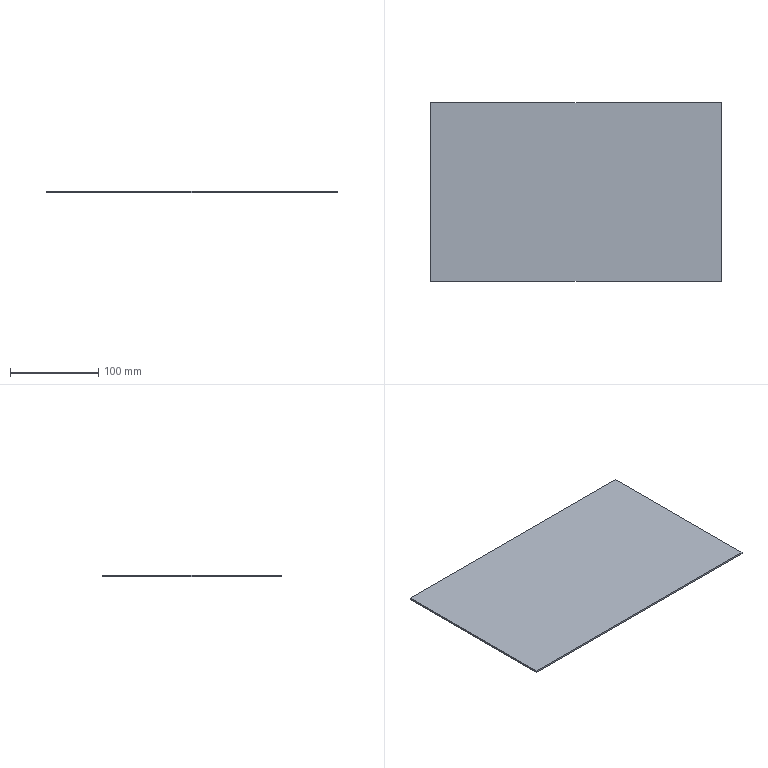Part | SolidWorks | features Extrusion 1 | 1 solid | 6 faces | box 330.2 x 203.2 x 2 mm | volume 134193 mm3 | plane 6
STEP:
#1=CARTESIAN_POINT('',(-165.1,101.6,-1.));
#2=VERTEX_POINT('',#1);
#3=CARTESIAN_POINT('',(-165.1,-101.6,-1.));
#4=VERTEX_POINT('',#3);
#5=CARTESIAN_POINT('',(-165.1,101.6,-1.));
#6=DIRECTION('',(0.,-1.,0.));
#7=VECTOR('',#6,1000.);
#8=LINE('',#5,#7);
#9=EDGE_CURVE('',#2,#4,#8,.T.);
#10=ORIENTED_EDGE('',*,*,#9,.T.);
#11=CARTESIAN_POINT('',(-165.1,-101.6,1.));
#12=VERTEX_POINT('',#11);
#13=CARTESIAN_POINT('',(-165.1,-101.6,1.));
#14=DIRECTION('',(0.,0.,-1.));
#15=VECTOR('',#14,1000.);
#16=LINE('',#13,#15);
#17=EDGE_CURVE('',#12,#4,#16,.T.);
#18=ORIENTED_EDGE('',*,*,#17,.F.);
#19=CARTESIAN_POINT('',(-165.1,101.6,1.));
#20=VERTEX_POINT('',#19);
#21=CARTESIAN_POINT('',(-165.1,101.6,1.));
#22=DIRECTION('',(0.,-1.,0.));
#23=VECTOR('',#22,1000.);
#24=LINE('',#21,#23);
#25=EDGE_CURVE('',#20,#12,#24,.T.);
#26=ORIENTED_EDGE('',*,*,#25,.F.);
#27=CARTESIAN_POINT('',(-165.1,101.6,1.));
#28=DIRECTION('',(0.,0.,-1.));
#29=VECTOR('',#28,1000.);
#30=LINE('',#27,#29);
#31=EDGE_CURVE('',#20,#2,#30,.T.);
#32=ORIENTED_EDGE('',*,*,#31,.T.);
#33=EDGE_LOOP('',(#10,#18,#26,#32));
#34=FACE_OUTER_BOUND('',#33,.T.);
#35=CARTESIAN_POINT('',(-165.1,101.6,1.));
#36=DIRECTION('',(1.,0.,0.));
#37=DIRECTION('',(0.,0.,-1.));
#38=AXIS2_PLACEMENT_3D('',#35,#36,#37);
#39=PLANE('',#38);
#40=ADVANCED_FACE('',(#34),#39,.F.);
#41=CARTESIAN_POINT('',(165.1,-101.6,-1.));
#42=VERTEX_POINT('',#41);
#43=CARTESIAN_POINT('',(-165.1,-101.6,-1.));
#44=DIRECTION('',(1.,0.,0.));
#45=VECTOR('',#44,1000.);
#46=LINE('',#43,#45);
#47=EDGE_CURVE('',#4,#42,#46,.T.);
#48=ORIENTED_EDGE('',*,*,#47,.T.);
#49=CARTESIAN_POINT('',(165.1,-101.6,1.));
#50=VERTEX_POINT('',#49);
#51=CARTESIAN_POINT('',(165.1,-101.6,1.));
#52=DIRECTION('',(0.,0.,-1.));
#53=VECTOR('',#52,1000.);
#54=LINE('',#51,#53);
#55=EDGE_CURVE('',#50,#42,#54,.T.);
#56=ORIENTED_EDGE('',*,*,#55,.F.);
#57=CARTESIAN_POINT('',(-165.1,-101.6,1.));
#58=DIRECTION('',(1.,0.,0.));
#59=VECTOR('',#58,1000.);
#60=LINE('',#57,#59);
#61=EDGE_CURVE('',#12,#50,#60,.T.);
#62=ORIENTED_EDGE('',*,*,#61,.F.);
#63=ORIENTED_EDGE('',*,*,#17,.T.);
#64=EDGE_LOOP('',(#48,#56,#62,#63));
#65=FACE_OUTER_BOUND('',#64,.T.);
#66=CARTESIAN_POINT('',(-165.1,-101.6,1.));
#67=DIRECTION('',(0.,1.,0.));
#68=DIRECTION('',(0.,0.,1.));
#69=AXIS2_PLACEMENT_3D('',#66,#67,#68);
#70=PLANE('',#69);
#71=ADVANCED_FACE('',(#65),#70,.F.);
#72=CARTESIAN_POINT('',(165.1,101.6,-1.));
#73=VERTEX_POINT('',#72);
#74=CARTESIAN_POINT('',(165.1,101.6,-1.));
#75=DIRECTION('',(0.,1.,0.));
#76=VECTOR('',#75,1000.);
#77=LINE('',#74,#76);
#78=EDGE_CURVE('',#42,#73,#77,.T.);
#79=ORIENTED_EDGE('',*,*,#78,.T.);
#80=CARTESIAN_POINT('',(165.1,101.6,1.));
#81=VERTEX_POINT('',#80);
#82=CARTESIAN_POINT('',(165.1,101.6,1.));
#83=DIRECTION('',(0.,0.,-1.));
#84=VECTOR('',#83,1000.);
#85=LINE('',#82,#84);
#86=EDGE_CURVE('',#81,#73,#85,.T.);
#87=ORIENTED_EDGE('',*,*,#86,.F.);
#88=CARTESIAN_POINT('',(165.1,101.6,1.));
#89=DIRECTION('',(0.,1.,0.));
#90=VECTOR('',#89,1000.);
#91=LINE('',#88,#90);
#92=EDGE_CURVE('',#50,#81,#91,.T.);
#93=ORIENTED_EDGE('',*,*,#92,.F.);
#94=ORIENTED_EDGE('',*,*,#55,.T.);
#95=EDGE_LOOP('',(#79,#87,#93,#94));
#96=FACE_OUTER_BOUND('',#95,.T.);
#97=CARTESIAN_POINT('',(165.1,101.6,1.));
#98=DIRECTION('',(-1.,0.,0.));
#99=DIRECTION('',(0.,-1.,0.));
#100=AXIS2_PLACEMENT_3D('',#97,#98,#99);
#101=PLANE('',#100);
#102=ADVANCED_FACE('',(#96),#101,.F.);
#103=CARTESIAN_POINT('',(-165.1,101.6,-1.));
#104=DIRECTION('',(-1.,0.,0.));
#105=VECTOR('',#104,1000.);
#106=LINE('',#103,#105);
#107=EDGE_CURVE('',#73,#2,#106,.T.);
#108=ORIENTED_EDGE('',*,*,#107,.T.);
#109=ORIENTED_EDGE('',*,*,#31,.F.);
#110=CARTESIAN_POINT('',(-165.1,101.6,1.));
#111=DIRECTION('',(-1.,0.,0.));
#112=VECTOR('',#111,1000.);
#113=LINE('',#110,#112);
#114=EDGE_CURVE('',#81,#20,#113,.T.);
#115=ORIENTED_EDGE('',*,*,#114,.F.);
#116=ORIENTED_EDGE('',*,*,#86,.T.);
#117=EDGE_LOOP('',(#108,#109,#115,#116));
#118=FACE_OUTER_BOUND('',#117,.T.);
#119=CARTESIAN_POINT('',(-165.1,101.6,1.));
#120=DIRECTION('',(0.,-1.,0.));
#121=DIRECTION('',(0.,0.,-1.));
#122=AXIS2_PLACEMENT_3D('',#119,#120,#121);
#123=PLANE('',#122);
#124=ADVANCED_FACE('',(#118),#123,.F.);
#125=ORIENTED_EDGE('',*,*,#25,.T.);
#126=ORIENTED_EDGE('',*,*,#61,.T.);
#127=ORIENTED_EDGE('',*,*,#92,.T.);
#128=ORIENTED_EDGE('',*,*,#114,.T.);
#129=EDGE_LOOP('',(#125,#126,#127,#128));
#130=FACE_OUTER_BOUND('',#129,.T.);
#131=CARTESIAN_POINT('',(0.,0.,1.));
#132=DIRECTION('',(0.,0.,1.));
#133=DIRECTION('',(1.,0.,0.));
#134=AXIS2_PLACEMENT_3D('',#131,#132,#133);
#135=PLANE('',#134);
#136=ADVANCED_FACE('',(#130),#135,.T.);
#137=ORIENTED_EDGE('',*,*,#9,.F.);
#138=ORIENTED_EDGE('',*,*,#107,.F.);
#139=ORIENTED_EDGE('',*,*,#78,.F.);
#140=ORIENTED_EDGE('',*,*,#47,.F.);
#141=EDGE_LOOP('',(#137,#138,#139,#140));
#142=FACE_OUTER_BOUND('',#141,.T.);
#143=CARTESIAN_POINT('',(0.,0.,-1.));
#144=DIRECTION('',(0.,0.,1.));
#145=DIRECTION('',(1.,0.,0.));
#146=AXIS2_PLACEMENT_3D('',#143,#144,#145);
#147=PLANE('',#146);
#148=ADVANCED_FACE('',(#142),#147,.F.);
#149=CLOSED_SHELL('',(#40,#71,#102,#124,#136,#148));
#150=MANIFOLD_SOLID_BREP('',#149);
#151=CARTESIAN_POINT('',(0.,0.,0.));
#152=DIRECTION('',(0.,0.,1.));
#153=DIRECTION('',(1.,0.,0.));
#154=AXIS2_PLACEMENT_3D('',#151,#152,#153);
#155=(LENGTH_UNIT()NAMED_UNIT(*)SI_UNIT(.MILLI.,.METRE.));
#156=UNCERTAINTY_MEASURE_WITH_UNIT(LENGTH_MEASURE(0.00001),#155,'','');
#157=(NAMED_UNIT(*)PLANE_ANGLE_UNIT()SI_UNIT($,.RADIAN.));
#158=(NAMED_UNIT(*)SI_UNIT($,.STERADIAN.)SOLID_ANGLE_UNIT());
#159=(GEOMETRIC_REPRESENTATION_CONTEXT(3)GLOBAL_UNCERTAINTY_ASSIGNED_CONTEXT((#156))GLOBAL_UNIT_ASSIGNED_CONTEXT((#155,#157,#158))REPRESENTATION_CONTEXT('',''));
#160=ADVANCED_BREP_SHAPE_REPRESENTATION('',(#150,#154),#159);